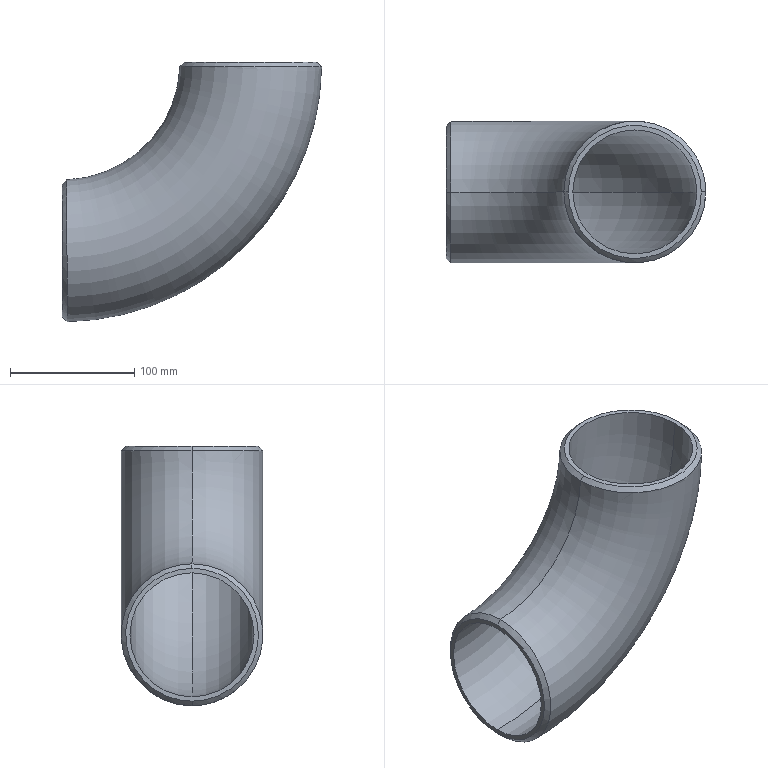Part | SolidWorks | features Chamfer 1, Revolution 1 | 1 solid | 10 faces | box 209.12 x 114.3 x 209.115 mm | volume 569487 mm3 | spline 4 | torus 4 | plane 2